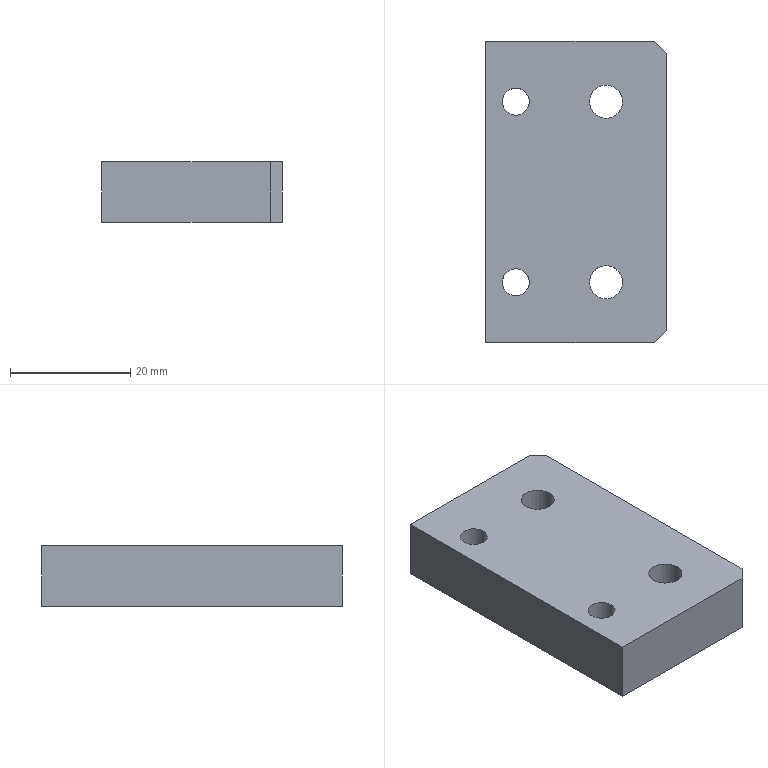Part | STEP file | 2094 Cylinder support base plate | 1 solid | 22 faces | box 30 x 50 x 10 mm | volume 13851 mm3 | cylinder 12 | plane 10 | commonest cylinder face diameters 4.5 x4 5.5 x4 8 x4